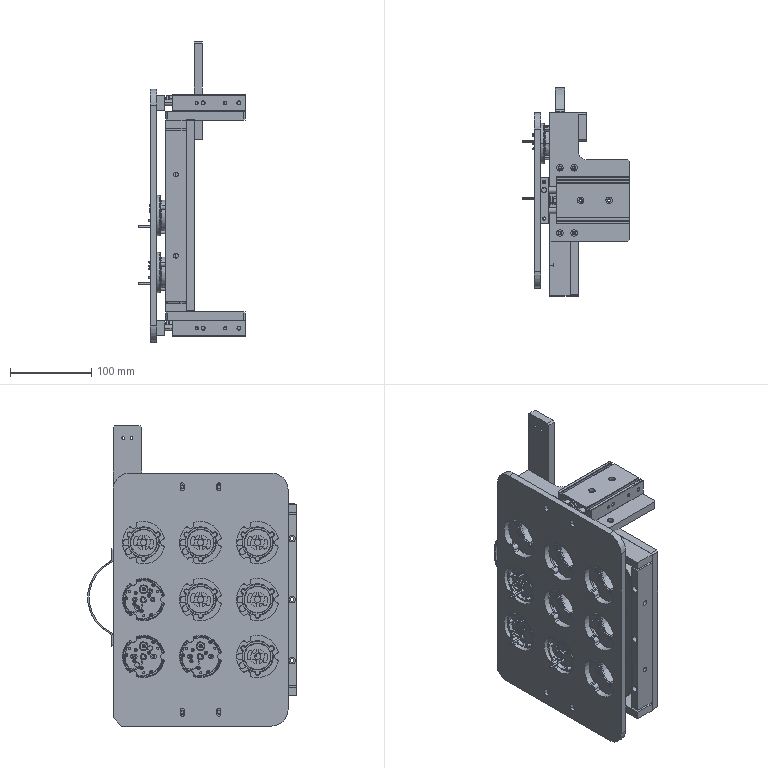Part | SolidWorks | features InContextFeatHolder 23, LocalLPattern 2, ReferencePattern 2 | 53 solids | 5415 faces | volume 4562071 mm3 | cylinder 1945 | plane 1863 | cone 1479 | spline 114 | torus 14 | commonest cylinder face diameters 4 x319 8 x122 5 x112 4.5 x102 7 x78 2 x68